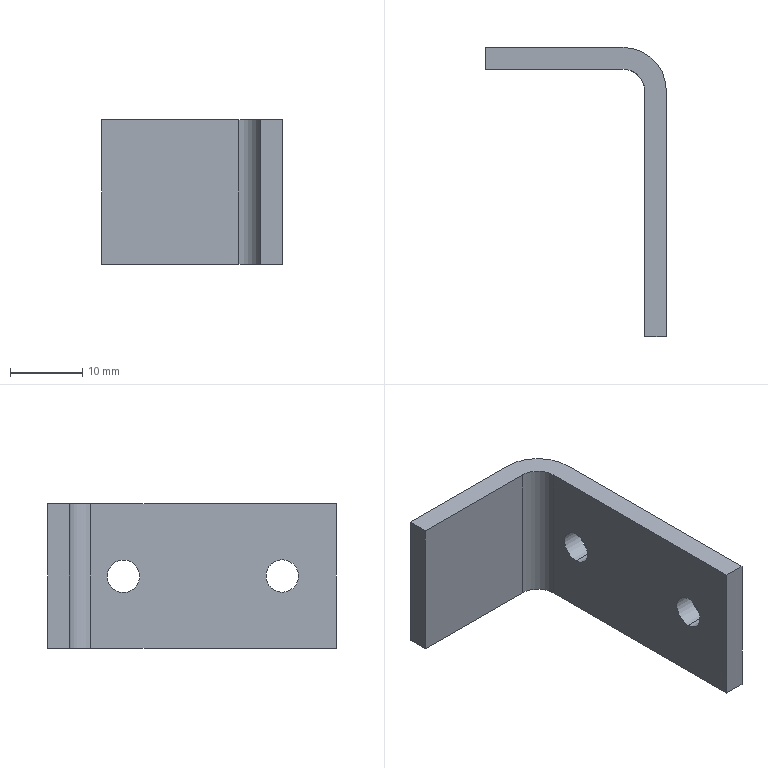Part | STEP file | X77-04019 | 1 solid | 14 faces | box 25 x 40 x 20 mm | volume 3509 mm3 | plane 8 | cylinder 6 | commonest cylinder face diameters 4.5 x4 6 x1 12 x1
STEP:
#1=CARTESIAN_POINT('',(-36.443,201.927,12.208));
#2=VERTEX_POINT('',#1);
#3=CARTESIAN_POINT('',(-36.443,201.927,7.708));
#4=VERTEX_POINT('',#3);
#5=CARTESIAN_POINT('',(-36.443,201.927,9.958));
#6=DIRECTION('',(1.,0.,0.));
#7=DIRECTION('',(0.,1.,0.));
#8=AXIS2_PLACEMENT_3D('',#5,#6,#7);
#9=CIRCLE('',#8,2.25);
#10=EDGE_CURVE('',#2,#4,#9,.T.);
#11=ORIENTED_EDGE('',*,*,#10,.F.);
#12=CARTESIAN_POINT('',(-33.443,201.927,12.208));
#13=VERTEX_POINT('',#12);
#14=CARTESIAN_POINT('',(-58.443,201.927,12.208));
#15=DIRECTION('',(1.,0.,0.));
#16=VECTOR('',#15,1000.);
#17=LINE('',#14,#16);
#18=EDGE_CURVE('',#2,#13,#17,.T.);
#19=ORIENTED_EDGE('',*,*,#18,.T.);
#20=CARTESIAN_POINT('',(-33.443,201.927,7.708));
#21=VERTEX_POINT('',#20);
#22=CARTESIAN_POINT('',(-33.443,201.927,9.958));
#23=DIRECTION('',(1.,0.,0.));
#24=DIRECTION('',(0.,0.,-1.));
#25=AXIS2_PLACEMENT_3D('',#22,#23,#24);
#26=CIRCLE('',#25,2.25);
#27=EDGE_CURVE('',#13,#21,#26,.T.);
#28=ORIENTED_EDGE('',*,*,#27,.T.);
#29=CARTESIAN_POINT('',(-58.443,201.927,7.708));
#30=DIRECTION('',(1.,0.,0.));
#31=VECTOR('',#30,1000.);
#32=LINE('',#29,#31);
#33=EDGE_CURVE('',#4,#21,#32,.T.);
#34=ORIENTED_EDGE('',*,*,#33,.F.);
#35=EDGE_LOOP('',(#11,#19,#28,#34));
#36=FACE_OUTER_BOUND('',#35,.T.);
#37=CARTESIAN_POINT('',(-58.443,201.927,9.958));
#38=DIRECTION('',(1.,0.,0.));
#39=DIRECTION('',(0.,0.,-1.));
#40=AXIS2_PLACEMENT_3D('',#37,#38,#39);
#41=CYLINDRICAL_SURFACE('',#40,2.25);
#42=ADVANCED_FACE('',(#36),#41,.F.);
#43=CARTESIAN_POINT('',(-36.443,179.927,12.25));
#44=VERTEX_POINT('',#43);
#45=CARTESIAN_POINT('',(-36.443,179.927,7.75));
#46=VERTEX_POINT('',#45);
#47=CARTESIAN_POINT('',(-36.443,179.927,10.));
#48=DIRECTION('',(1.,0.,0.));
#49=DIRECTION('',(0.,1.,0.));
#50=AXIS2_PLACEMENT_3D('',#47,#48,#49);
#51=CIRCLE('',#50,2.25);
#52=EDGE_CURVE('',#44,#46,#51,.T.);
#53=ORIENTED_EDGE('',*,*,#52,.F.);
#54=CARTESIAN_POINT('',(-33.443,179.927,12.25));
#55=VERTEX_POINT('',#54);
#56=CARTESIAN_POINT('',(-58.443,179.927,12.25));
#57=DIRECTION('',(1.,0.,0.));
#58=VECTOR('',#57,1000.);
#59=LINE('',#56,#58);
#60=EDGE_CURVE('',#44,#55,#59,.T.);
#61=ORIENTED_EDGE('',*,*,#60,.T.);
#62=CARTESIAN_POINT('',(-33.443,179.927,7.75));
#63=VERTEX_POINT('',#62);
#64=CARTESIAN_POINT('',(-33.443,179.927,10.));
#65=DIRECTION('',(1.,0.,0.));
#66=DIRECTION('',(0.,0.,-1.));
#67=AXIS2_PLACEMENT_3D('',#64,#65,#66);
#68=CIRCLE('',#67,2.25);
#69=EDGE_CURVE('',#55,#63,#68,.T.);
#70=ORIENTED_EDGE('',*,*,#69,.T.);
#71=CARTESIAN_POINT('',(-58.443,179.927,7.75));
#72=DIRECTION('',(1.,0.,0.));
#73=VECTOR('',#72,1000.);
#74=LINE('',#71,#73);
#75=EDGE_CURVE('',#46,#63,#74,.T.);
#76=ORIENTED_EDGE('',*,*,#75,.F.);
#77=EDGE_LOOP('',(#53,#61,#70,#76));
#78=FACE_OUTER_BOUND('',#77,.T.);
#79=CARTESIAN_POINT('',(-58.443,179.927,10.));
#80=DIRECTION('',(1.,0.,0.));
#81=DIRECTION('',(0.,0.,-1.));
#82=AXIS2_PLACEMENT_3D('',#79,#80,#81);
#83=CYLINDRICAL_SURFACE('',#82,2.25);
#84=ADVANCED_FACE('',(#78),#83,.F.);
#85=CARTESIAN_POINT('',(-33.443,201.927,9.958));
#86=DIRECTION('',(1.,0.,0.));
#87=DIRECTION('',(0.,0.,-1.));
#88=AXIS2_PLACEMENT_3D('',#85,#86,#87);
#89=CIRCLE('',#88,2.25);
#90=EDGE_CURVE('',#21,#13,#89,.T.);
#91=ORIENTED_EDGE('',*,*,#90,.F.);
#92=ORIENTED_EDGE('',*,*,#27,.F.);
#93=EDGE_LOOP('',(#91,#92));
#94=FACE_BOUND('',#93,.T.);
#95=CARTESIAN_POINT('',(-33.443,179.927,10.));
#96=DIRECTION('',(1.,0.,0.));
#97=DIRECTION('',(0.,0.,-1.));
#98=AXIS2_PLACEMENT_3D('',#95,#96,#97);
#99=CIRCLE('',#98,2.25);
#100=EDGE_CURVE('',#63,#55,#99,.T.);
#101=ORIENTED_EDGE('',*,*,#100,.F.);
#102=ORIENTED_EDGE('',*,*,#69,.F.);
#103=EDGE_LOOP('',(#101,#102));
#104=FACE_BOUND('',#103,.T.);
#105=CARTESIAN_POINT('',(-33.443,172.427,0.));
#106=VERTEX_POINT('',#105);
#107=CARTESIAN_POINT('',(-33.443,206.427,0.));
#108=VERTEX_POINT('',#107);
#109=CARTESIAN_POINT('',(-33.443,172.427,0.));
#110=DIRECTION('',(0.,1.,0.));
#111=VECTOR('',#110,1000.);
#112=LINE('',#109,#111);
#113=EDGE_CURVE('',#106,#108,#112,.T.);
#114=ORIENTED_EDGE('',*,*,#113,.T.);
#115=CARTESIAN_POINT('',(-33.443,206.427,20.));
#116=VERTEX_POINT('',#115);
#117=CARTESIAN_POINT('',(-33.443,206.427,20.));
#118=DIRECTION('',(0.,0.,1.));
#119=VECTOR('',#118,1000.);
#120=LINE('',#117,#119);
#121=EDGE_CURVE('',#108,#116,#120,.T.);
#122=ORIENTED_EDGE('',*,*,#121,.T.);
#123=CARTESIAN_POINT('',(-33.443,172.427,20.));
#124=VERTEX_POINT('',#123);
#125=CARTESIAN_POINT('',(-33.443,172.427,20.));
#126=DIRECTION('',(0.,1.,0.));
#127=VECTOR('',#126,1000.);
#128=LINE('',#125,#127);
#129=EDGE_CURVE('',#124,#116,#128,.T.);
#130=ORIENTED_EDGE('',*,*,#129,.F.);
#131=CARTESIAN_POINT('',(-33.443,172.427,20.));
#132=DIRECTION('',(0.,0.,-1.));
#133=VECTOR('',#132,1000.);
#134=LINE('',#131,#133);
#135=EDGE_CURVE('',#124,#106,#134,.T.);
#136=ORIENTED_EDGE('',*,*,#135,.T.);
#137=EDGE_LOOP('',(#114,#122,#130,#136));
#138=FACE_OUTER_BOUND('',#137,.T.);
#139=CARTESIAN_POINT('',(-33.443,172.427,20.));
#140=DIRECTION('',(-1.,0.,0.));
#141=DIRECTION('',(0.,0.,1.));
#142=AXIS2_PLACEMENT_3D('',#139,#140,#141);
#143=PLANE('',#142);
#144=ADVANCED_FACE('',(#94,#104,#138),#143,.F.);
#145=CARTESIAN_POINT('',(-39.443,212.427,20.));
#146=VERTEX_POINT('',#145);
#147=CARTESIAN_POINT('',(-58.443,212.427,20.));
#148=VERTEX_POINT('',#147);
#149=CARTESIAN_POINT('',(-33.443,212.427,20.));
#150=DIRECTION('',(-1.,0.,0.));
#151=VECTOR('',#150,1000.);
#152=LINE('',#149,#151);
#153=EDGE_CURVE('',#146,#148,#152,.T.);
#154=ORIENTED_EDGE('',*,*,#153,.F.);
#155=CARTESIAN_POINT('',(-39.443,212.427,0.));
#156=VERTEX_POINT('',#155);
#157=CARTESIAN_POINT('',(-39.443,212.427,20.));
#158=DIRECTION('',(0.,0.,-1.));
#159=VECTOR('',#158,1000.);
#160=LINE('',#157,#159);
#161=EDGE_CURVE('',#146,#156,#160,.T.);
#162=ORIENTED_EDGE('',*,*,#161,.T.);
#163=CARTESIAN_POINT('',(-58.443,212.427,0.));
#164=VERTEX_POINT('',#163);
#165=CARTESIAN_POINT('',(-33.443,212.427,0.));
#166=DIRECTION('',(-1.,0.,0.));
#167=VECTOR('',#166,1000.);
#168=LINE('',#165,#167);
#169=EDGE_CURVE('',#156,#164,#168,.T.);
#170=ORIENTED_EDGE('',*,*,#169,.T.);
#171=CARTESIAN_POINT('',(-58.443,212.427,20.));
#172=DIRECTION('',(0.,0.,-1.));
#173=VECTOR('',#172,1000.);
#174=LINE('',#171,#173);
#175=EDGE_CURVE('',#148,#164,#174,.T.);
#176=ORIENTED_EDGE('',*,*,#175,.F.);
#177=EDGE_LOOP('',(#154,#162,#170,#176));
#178=FACE_OUTER_BOUND('',#177,.T.);
#179=CARTESIAN_POINT('',(-33.443,212.427,20.));
#180=DIRECTION('',(0.,-1.,0.));
#181=DIRECTION('',(0.,0.,-1.));
#182=AXIS2_PLACEMENT_3D('',#179,#180,#181);
#183=PLANE('',#182);
#184=ADVANCED_FACE('',(#178),#183,.F.);
#185=CARTESIAN_POINT('',(-58.443,209.427,0.));
#186=VERTEX_POINT('',#185);
#187=CARTESIAN_POINT('',(-58.443,212.427,0.));
#188=DIRECTION('',(0.,-1.,0.));
#189=VECTOR('',#188,1000.);
#190=LINE('',#187,#189);
#191=EDGE_CURVE('',#164,#186,#190,.T.);
#192=ORIENTED_EDGE('',*,*,#191,.T.);
#193=CARTESIAN_POINT('',(-58.443,209.427,20.));
#194=VERTEX_POINT('',#193);
#195=CARTESIAN_POINT('',(-58.443,209.427,20.));
#196=DIRECTION('',(0.,0.,-1.));
#197=VECTOR('',#196,1000.);
#198=LINE('',#195,#197);
#199=EDGE_CURVE('',#194,#186,#198,.T.);
#200=ORIENTED_EDGE('',*,*,#199,.F.);
#201=CARTESIAN_POINT('',(-58.443,212.427,20.));
#202=DIRECTION('',(0.,-1.,0.));
#203=VECTOR('',#202,1000.);
#204=LINE('',#201,#203);
#205=EDGE_CURVE('',#148,#194,#204,.T.);
#206=ORIENTED_EDGE('',*,*,#205,.F.);
#207=ORIENTED_EDGE('',*,*,#175,.T.);
#208=EDGE_LOOP('',(#192,#200,#206,#207));
#209=FACE_OUTER_BOUND('',#208,.T.);
#210=CARTESIAN_POINT('',(-58.443,212.427,20.));
#211=DIRECTION('',(1.,0.,0.));
#212=DIRECTION('',(0.,0.,-1.));
#213=AXIS2_PLACEMENT_3D('',#210,#211,#212);
#214=PLANE('',#213);
#215=ADVANCED_FACE('',(#209),#214,.F.);
#216=CARTESIAN_POINT('',(-39.443,209.427,0.));
#217=VERTEX_POINT('',#216);
#218=CARTESIAN_POINT('',(-58.443,209.427,0.));
#219=DIRECTION('',(1.,0.,0.));
#220=VECTOR('',#219,1000.);
#221=LINE('',#218,#220);
#222=EDGE_CURVE('',#186,#217,#221,.T.);
#223=ORIENTED_EDGE('',*,*,#222,.T.);
#224=CARTESIAN_POINT('',(-39.443,209.427,20.));
#225=VERTEX_POINT('',#224);
#226=CARTESIAN_POINT('',(-39.443,209.427,20.));
#227=DIRECTION('',(0.,0.,1.));
#228=VECTOR('',#227,1000.);
#229=LINE('',#226,#228);
#230=EDGE_CURVE('',#217,#225,#229,.T.);
#231=ORIENTED_EDGE('',*,*,#230,.T.);
#232=CARTESIAN_POINT('',(-58.443,209.427,20.));
#233=DIRECTION('',(1.,0.,0.));
#234=VECTOR('',#233,1000.);
#235=LINE('',#232,#234);
#236=EDGE_CURVE('',#194,#225,#235,.T.);
#237=ORIENTED_EDGE('',*,*,#236,.F.);
#238=ORIENTED_EDGE('',*,*,#199,.T.);
#239=EDGE_LOOP('',(#223,#231,#237,#238));
#240=FACE_OUTER_BOUND('',#239,.T.);
#241=CARTESIAN_POINT('',(-58.443,209.427,20.));
#242=DIRECTION('',(0.,1.,0.));
#243=DIRECTION('',(0.,0.,1.));
#244=AXIS2_PLACEMENT_3D('',#241,#242,#243);
#245=PLANE('',#244);
#246=ADVANCED_FACE('',(#240),#245,.F.);
#247=CARTESIAN_POINT('',(-36.443,201.927,9.958));
#248=DIRECTION('',(1.,0.,0.));
#249=DIRECTION('',(0.,1.,0.));
#250=AXIS2_PLACEMENT_3D('',#247,#248,#249);
#251=CIRCLE('',#250,2.25);
#252=EDGE_CURVE('',#4,#2,#251,.T.);
#253=ORIENTED_EDGE('',*,*,#252,.T.);
#254=ORIENTED_EDGE('',*,*,#10,.T.);
#255=EDGE_LOOP('',(#253,#254));
#256=FACE_BOUND('',#255,.T.);
#257=CARTESIAN_POINT('',(-36.443,179.927,10.));
#258=DIRECTION('',(1.,0.,0.));
#259=DIRECTION('',(0.,1.,0.));
#260=AXIS2_PLACEMENT_3D('',#257,#258,#259);
#261=CIRCLE('',#260,2.25);
#262=EDGE_CURVE('',#46,#44,#261,.T.);
#263=ORIENTED_EDGE('',*,*,#262,.T.);
#264=ORIENTED_EDGE('',*,*,#52,.T.);
#265=EDGE_LOOP('',(#263,#264));
#266=FACE_BOUND('',#265,.T.);
#267=CARTESIAN_POINT('',(-36.443,206.427,20.));
#268=VERTEX_POINT('',#267);
#269=CARTESIAN_POINT('',(-36.443,172.427,20.));
#270=VERTEX_POINT('',#269);
#271=CARTESIAN_POINT('',(-36.443,209.427,20.));
#272=DIRECTION('',(0.,-1.,0.));
#273=VECTOR('',#272,1000.);
#274=LINE('',#271,#273);
#275=EDGE_CURVE('',#268,#270,#274,.T.);
#276=ORIENTED_EDGE('',*,*,#275,.F.);
#277=CARTESIAN_POINT('',(-36.443,206.427,0.));
#278=VERTEX_POINT('',#277);
#279=CARTESIAN_POINT('',(-36.443,206.427,0.));
#280=DIRECTION('',(0.,0.,-1.));
#281=VECTOR('',#280,1000.);
#282=LINE('',#279,#281);
#283=EDGE_CURVE('',#268,#278,#282,.T.);
#284=ORIENTED_EDGE('',*,*,#283,.T.);
#285=CARTESIAN_POINT('',(-36.443,172.427,0.));
#286=VERTEX_POINT('',#285);
#287=CARTESIAN_POINT('',(-36.443,209.427,0.));
#288=DIRECTION('',(0.,-1.,0.));
#289=VECTOR('',#288,1000.);
#290=LINE('',#287,#289);
#291=EDGE_CURVE('',#278,#286,#290,.T.);
#292=ORIENTED_EDGE('',*,*,#291,.T.);
#293=CARTESIAN_POINT('',(-36.443,172.427,20.));
#294=DIRECTION('',(0.,0.,-1.));
#295=VECTOR('',#294,1000.);
#296=LINE('',#293,#295);
#297=EDGE_CURVE('',#270,#286,#296,.T.);
#298=ORIENTED_EDGE('',*,*,#297,.F.);
#299=EDGE_LOOP('',(#276,#284,#292,#298));
#300=FACE_OUTER_BOUND('',#299,.T.);
#301=CARTESIAN_POINT('',(-36.443,209.427,20.));
#302=DIRECTION('',(1.,0.,0.));
#303=DIRECTION('',(0.,1.,0.));
#304=AXIS2_PLACEMENT_3D('',#301,#302,#303);
#305=PLANE('',#304);
#306=ADVANCED_FACE('',(#256,#266,#300),#305,.F.);
#307=CARTESIAN_POINT('',(-36.443,172.427,0.));
#308=DIRECTION('',(1.,0.,0.));
#309=VECTOR('',#308,1000.);
#310=LINE('',#307,#309);
#311=EDGE_CURVE('',#286,#106,#310,.T.);
#312=ORIENTED_EDGE('',*,*,#311,.T.);
#313=ORIENTED_EDGE('',*,*,#135,.F.);
#314=CARTESIAN_POINT('',(-36.443,172.427,20.));
#315=DIRECTION('',(1.,0.,0.));
#316=VECTOR('',#315,1000.);
#317=LINE('',#314,#316);
#318=EDGE_CURVE('',#270,#124,#317,.T.);
#319=ORIENTED_EDGE('',*,*,#318,.F.);
#320=ORIENTED_EDGE('',*,*,#297,.T.);
#321=EDGE_LOOP('',(#312,#313,#319,#320));
#322=FACE_OUTER_BOUND('',#321,.T.);
#323=CARTESIAN_POINT('',(-36.443,172.427,20.));
#324=DIRECTION('',(0.,1.,0.));
#325=DIRECTION('',(0.,0.,1.));
#326=AXIS2_PLACEMENT_3D('',#323,#324,#325);
#327=PLANE('',#326);
#328=ADVANCED_FACE('',(#322),#327,.F.);
#329=ORIENTED_EDGE('',*,*,#129,.T.);
#330=CARTESIAN_POINT('',(-39.443,206.427,20.));
#331=DIRECTION('',(0.,0.,1.));
#332=DIRECTION('',(1.,0.,0.));
#333=AXIS2_PLACEMENT_3D('',#330,#331,#332);
#334=CIRCLE('',#333,6.);
#335=EDGE_CURVE('',#116,#146,#334,.T.);
#336=ORIENTED_EDGE('',*,*,#335,.T.);
#337=ORIENTED_EDGE('',*,*,#153,.T.);
#338=ORIENTED_EDGE('',*,*,#205,.T.);
#339=ORIENTED_EDGE('',*,*,#236,.T.);
#340=CARTESIAN_POINT('',(-39.443,206.427,20.));
#341=DIRECTION('',(0.,0.,-1.));
#342=DIRECTION('',(1.,0.,0.));
#343=AXIS2_PLACEMENT_3D('',#340,#341,#342);
#344=CIRCLE('',#343,3.);
#345=EDGE_CURVE('',#225,#268,#344,.T.);
#346=ORIENTED_EDGE('',*,*,#345,.T.);
#347=ORIENTED_EDGE('',*,*,#275,.T.);
#348=ORIENTED_EDGE('',*,*,#318,.T.);
#349=EDGE_LOOP('',(#329,#336,#337,#338,#339,#346,#347,#348));
#350=FACE_OUTER_BOUND('',#349,.T.);
#351=CARTESIAN_POINT('',(-33.443,212.427,20.));
#352=DIRECTION('',(0.,0.,1.));
#353=DIRECTION('',(1.,0.,0.));
#354=AXIS2_PLACEMENT_3D('',#351,#352,#353);
#355=PLANE('',#354);
#356=ADVANCED_FACE('',(#350),#355,.T.);
#357=ORIENTED_EDGE('',*,*,#169,.F.);
#358=CARTESIAN_POINT('',(-39.443,206.427,0.));
#359=DIRECTION('',(0.,0.,-1.));
#360=DIRECTION('',(1.,0.,0.));
#361=AXIS2_PLACEMENT_3D('',#358,#359,#360);
#362=CIRCLE('',#361,6.);
#363=EDGE_CURVE('',#156,#108,#362,.T.);
#364=ORIENTED_EDGE('',*,*,#363,.T.);
#365=ORIENTED_EDGE('',*,*,#113,.F.);
#366=ORIENTED_EDGE('',*,*,#311,.F.);
#367=ORIENTED_EDGE('',*,*,#291,.F.);
#368=CARTESIAN_POINT('',(-39.443,206.427,0.));
#369=DIRECTION('',(0.,0.,1.));
#370=DIRECTION('',(1.,0.,0.));
#371=AXIS2_PLACEMENT_3D('',#368,#369,#370);
#372=CIRCLE('',#371,3.);
#373=EDGE_CURVE('',#278,#217,#372,.T.);
#374=ORIENTED_EDGE('',*,*,#373,.T.);
#375=ORIENTED_EDGE('',*,*,#222,.F.);
#376=ORIENTED_EDGE('',*,*,#191,.F.);
#377=EDGE_LOOP('',(#357,#364,#365,#366,#367,#374,#375,#376));
#378=FACE_OUTER_BOUND('',#377,.T.);
#379=CARTESIAN_POINT('',(-33.443,212.427,0.));
#380=DIRECTION('',(0.,0.,1.));
#381=DIRECTION('',(1.,0.,0.));
#382=AXIS2_PLACEMENT_3D('',#379,#380,#381);
#383=PLANE('',#382);
#384=ADVANCED_FACE('',(#378),#383,.F.);
#385=ORIENTED_EDGE('',*,*,#60,.F.);
#386=ORIENTED_EDGE('',*,*,#262,.F.);
#387=ORIENTED_EDGE('',*,*,#75,.T.);
#388=ORIENTED_EDGE('',*,*,#100,.T.);
#389=EDGE_LOOP('',(#385,#386,#387,#388));
#390=FACE_OUTER_BOUND('',#389,.T.);
#391=CARTESIAN_POINT('',(-58.443,179.927,10.));
#392=DIRECTION('',(1.,0.,0.));
#393=DIRECTION('',(0.,0.,-1.));
#394=AXIS2_PLACEMENT_3D('',#391,#392,#393);
#395=CYLINDRICAL_SURFACE('',#394,2.25);
#396=ADVANCED_FACE('',(#390),#395,.F.);
#397=ORIENTED_EDGE('',*,*,#18,.F.);
#398=ORIENTED_EDGE('',*,*,#252,.F.);
#399=ORIENTED_EDGE('',*,*,#33,.T.);
#400=ORIENTED_EDGE('',*,*,#90,.T.);
#401=EDGE_LOOP('',(#397,#398,#399,#400));
#402=FACE_OUTER_BOUND('',#401,.T.);
#403=CARTESIAN_POINT('',(-58.443,201.927,9.958));
#404=DIRECTION('',(1.,0.,0.));
#405=DIRECTION('',(0.,0.,-1.));
#406=AXIS2_PLACEMENT_3D('',#403,#404,#405);
#407=CYLINDRICAL_SURFACE('',#406,2.25);
#408=ADVANCED_FACE('',(#402),#407,.F.);
#409=ORIENTED_EDGE('',*,*,#345,.F.);
#410=ORIENTED_EDGE('',*,*,#230,.F.);
#411=ORIENTED_EDGE('',*,*,#373,.F.);
#412=ORIENTED_EDGE('',*,*,#283,.F.);
#413=EDGE_LOOP('',(#409,#410,#411,#412));
#414=FACE_OUTER_BOUND('',#413,.T.);
#415=CARTESIAN_POINT('',(-39.443,206.427,20.));
#416=DIRECTION('',(0.,0.,1.));
#417=DIRECTION('',(1.,0.,0.));
#418=AXIS2_PLACEMENT_3D('',#415,#416,#417);
#419=CYLINDRICAL_SURFACE('',#418,3.);
#420=ADVANCED_FACE('',(#414),#419,.F.);
#421=ORIENTED_EDGE('',*,*,#335,.F.);
#422=ORIENTED_EDGE('',*,*,#121,.F.);
#423=ORIENTED_EDGE('',*,*,#363,.F.);
#424=ORIENTED_EDGE('',*,*,#161,.F.);
#425=EDGE_LOOP('',(#421,#422,#423,#424));
#426=FACE_OUTER_BOUND('',#425,.T.);
#427=CARTESIAN_POINT('',(-39.443,206.427,20.));
#428=DIRECTION('',(0.,0.,-1.));
#429=DIRECTION('',(-1.,0.,0.));
#430=AXIS2_PLACEMENT_3D('',#427,#428,#429);
#431=CYLINDRICAL_SURFACE('',#430,6.);
#432=ADVANCED_FACE('',(#426),#431,.T.);
#433=CLOSED_SHELL('',(#42,#84,#144,#184,#215,#246,#306,#328,#356,#384,#396,#408,#420,#432));
#434=MANIFOLD_SOLID_BREP('',#433);
#435=CARTESIAN_POINT('',(0.,0.,0.));
#436=DIRECTION('',(0.,0.,1.));
#437=DIRECTION('',(1.,0.,0.));
#438=AXIS2_PLACEMENT_3D('',#435,#436,#437);
#439=(LENGTH_UNIT()NAMED_UNIT(*)SI_UNIT(.MILLI.,.METRE.));
#440=UNCERTAINTY_MEASURE_WITH_UNIT(LENGTH_MEASURE(0.00001),#439,'','');
#441=(NAMED_UNIT(*)PLANE_ANGLE_UNIT()SI_UNIT($,.RADIAN.));
#442=(NAMED_UNIT(*)SI_UNIT($,.STERADIAN.)SOLID_ANGLE_UNIT());
#443=(GEOMETRIC_REPRESENTATION_CONTEXT(3)GLOBAL_UNCERTAINTY_ASSIGNED_CONTEXT((#440))GLOBAL_UNIT_ASSIGNED_CONTEXT((#439,#441,#442))REPRESENTATION_CONTEXT('',''));
#444=ADVANCED_BREP_SHAPE_REPRESENTATION('',(#434,#438),#443);